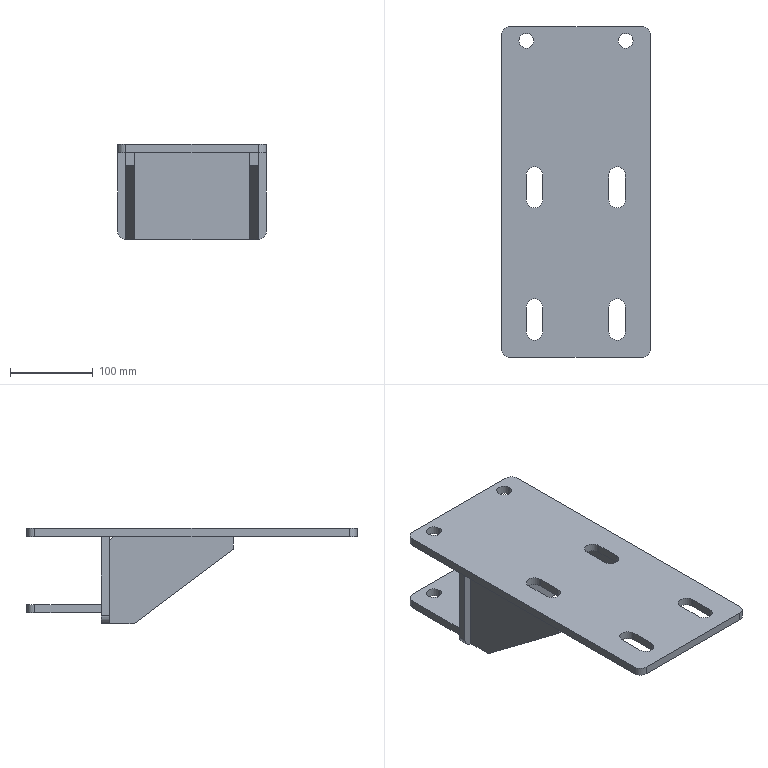Part | SolidWorks | features ICE 4, Fillet 3, Gusset 2, Extrusion 1, HoleWzd 1 | 5 solids | 66 faces | box 180 x 400 x 115 mm | volume 1229288 mm3 | plane 42 | cylinder 24 | commonest cylinder face diameters 20 x16 18 x8